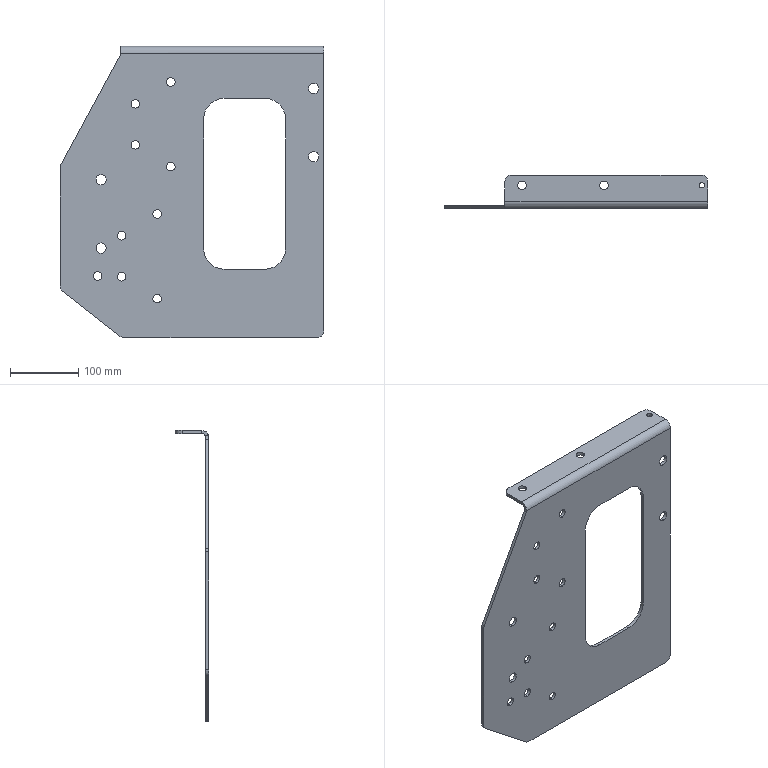Part | SolidWorks | features ICE 2, Fillet 1, FlatPattern 1, SMBaseFlange 1, SheetMetal 1 | 1 solid | 63 faces | box 386 x 49 x 426 mm | volume 601864 mm3 | cylinder 45 | plane 18 | commonest cylinder face diameters 12.5 x22 15 x8 20 x7 60 x4 8 x2 12 x1